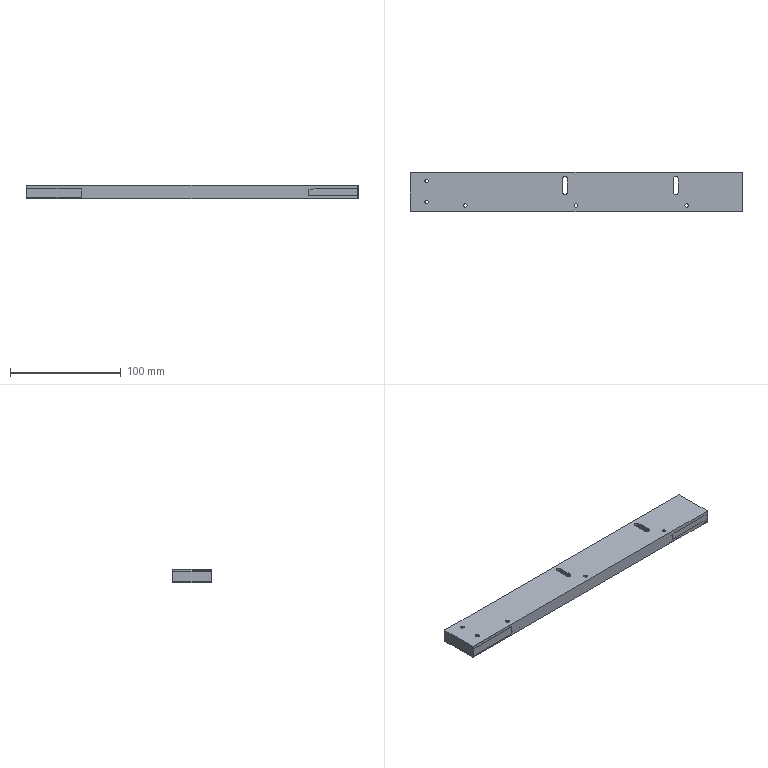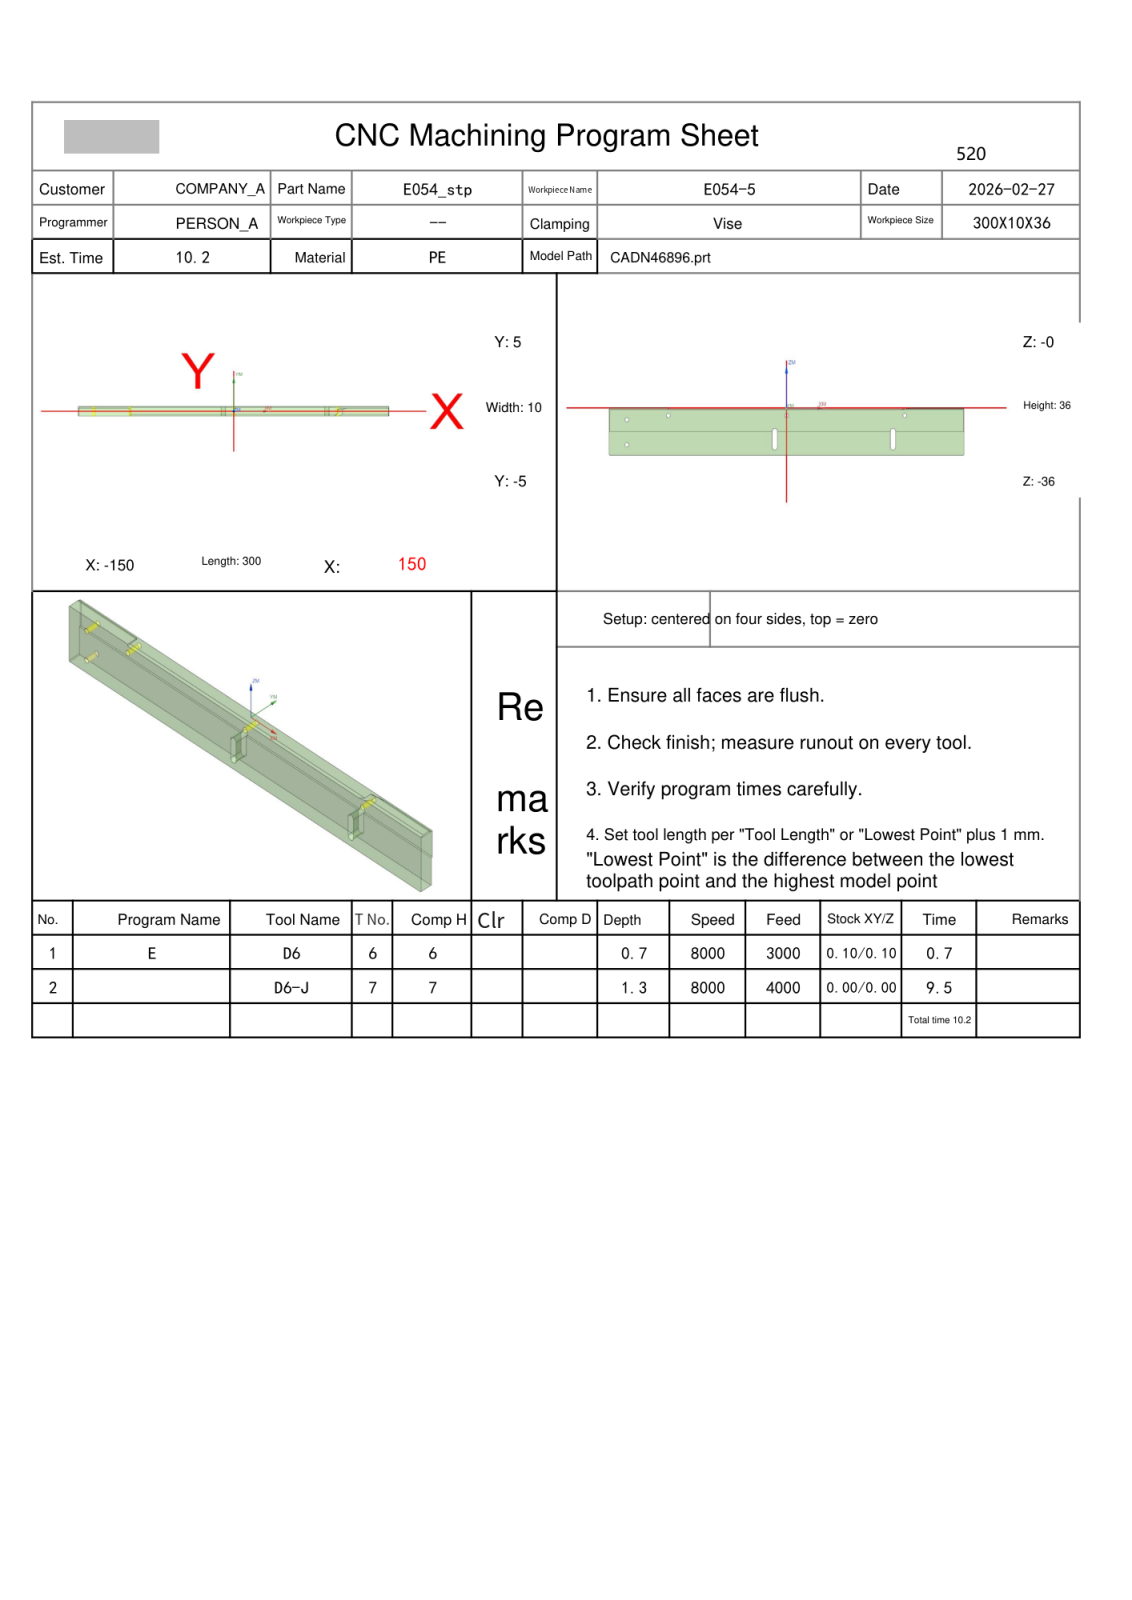NC program | NX | posted by the shop | part box 300 x 36 x 12 mm
Lines 117 to 1396 of 2760:
N2 T07 M06
(D6-J  D=6. R=0. H=07 ce=0.40 di=0.00)
G00 G90 G54 X-1.2 Y8.7 M03 S8000
G43 H07 Z10.4
M08
Z.7
G01 Z-.8 F1000.
Y6.3
G03 X0.0 Y5.1 I1.2 J0.0
G01 X98.232
X98.35 Y4.98
X98.29 Y4.876
X98.157 Y4.803
X97.117 Y3.838
X96.6 Y2.387
Y-3.004
G02 X96.004 Y-3.6 I-.6 J.004
G01 X-96.004
G02 X-96.6 Y-3.004 I.004 J.6
G01 Y4.504
G02 X-96.004 Y5.1 I.6 J-.004
G01 X1.252
G02 X1.675 Y4.925 I-.001 J-.6
G01 X4.325 Y2.275
G03 X4.748 Y2.1 I.424 J.425
G01 X93.004
G02 X93.6 Y1.504 I-.004 J-.6
G01 Y-.004
G02 X93.004 Y-.6 I-.6 J.004
G01 X-93.004
G02 X-93.6 Y-.004 I.004 J.6
G01 Y1.504
G02 X-93.004 Y2.1 I.6 J-.004
G01 X3.
X4.
G03 X5.2 Y3.3 I0.0 J1.2
G01 Y8.7
Z.7
G00 Z10.4
G00 G90 X-154.2 Y7.199 M03 S8000
Z11.2
Z.2
G01 Z-.8 F1000.
G41 D07
Y6.999
G03 X-153. Y5.8 I1.2 J.001
G01 X-97.
Y-6.
G03 X-95.8 Y-7.2 I1.2 J0.0
G01 G40 X-95.6
Z.2
G00 X95.6
G01 Z-.8
G41 D07
X95.8
G03 X97. Y-6. I0.0 J1.2
G01 Y2.09
X97.165 Y2.938
X97.648 Y3.76
X98.146 Y4.267
X98.579 Y4.58
X98.953 Y4.788
X99.287 Y4.938
G02 X100.818 Y5.37 I2.982 J-7.627
G01 X101.137 Y5.429
X101.467 Y5.483
G02 X103.27 Y5.686 I3.532 J-23.309
X106.21 Y5.8 I2.94 J-37.717
G01 X106.326
X153.
G03 X154.2 Y6.999 I0.0 J1.2
G01 G40 Y7.199
Z.2
G00 Z11.2
G00 G90 X96.912 Y-10.137 M03 S8000
Z10.01
Z-.304
G01 Z-.804 F4000.
X97.217 Y-6.067
X97.219 Y-6.025
X97.188 Y-5.992
X97.146 Y-5.99
X-97.151
X-97.176 Y-6.042
Z-.808
X97.127
X97.108 Y-6.058 Z-.812
X-97.182
X-97.188 Y-6.074 Z-.816
X97.089
X97.07 Y-6.09 Z-.82
X-97.194
X-97.201 Y-6.106 Z-.824
X97.051
X97.033 Y-6.122 Z-.828
X-97.207
X-97.213 Y-6.138 Z-.832
X97.015
X96.998 Y-6.154 Z-.836
X-97.22
X-97.227 Y-6.17 Z-.84
X96.98
X96.962 Y-6.186 Z-.844
X-97.234
X-97.24 Y-6.202 Z-.848
X96.945
X96.927 Y-6.218 Z-.852
X-97.247
X-97.255 Y-6.234 Z-.856
X96.91
X96.892 Y-6.25 Z-.86
X-97.262
X-97.269 Y-6.266 Z-.864
X96.875
X96.857 Y-6.282 Z-.868
X-97.277
X-97.284 Y-6.298 Z-.872
X96.84
X96.822 Y-6.314 Z-.876
X-97.292
X-97.3 Y-6.33 Z-.88
X96.805
X96.787 Y-6.346 Z-.884
X-97.308
X-97.316 Y-6.362 Z-.888
X96.769
X96.752 Y-6.378 Z-.892
X-97.324
X-97.332 Y-6.394 Z-.896
X96.734
X96.717 Y-6.41 Z-.9
X-97.341
X-97.349 Y-6.426 Z-.904
X96.7
X96.684 Y-6.442 Z-.908
X-97.358
X-97.367 Y-6.458 Z-.912
X96.668
X96.652 Y-6.474 Z-.916
X-97.376
X-97.385 Y-6.49 Z-.92
X96.637
X96.623 Y-6.506 Z-.924
X-97.394
X-97.403 Y-6.522 Z-.928
X96.608
X96.593 Y-6.538 Z-.932
X-97.413
X-97.422 Y-6.554 Z-.936
X96.579
X96.564 Y-6.57 Z-.94
X-97.432
X-97.442 Y-6.586 Z-.944
X96.549
X96.535 Y-6.602 Z-.948
X-97.452
X-97.462 Y-6.618 Z-.952
X96.52
X96.505 Y-6.634 Z-.956
X-97.472
X-97.483 Y-6.65 Z-.96
X96.49
X96.476 Y-6.666 Z-.964
X-97.493
X-97.504 Y-6.682 Z-.968
X96.461
X96.446 Y-6.698 Z-.972
X-97.515
X-97.526 Y-6.714 Z-.976
X96.432
X96.417 Y-6.73 Z-.98
X-97.537
X-97.548 Y-6.746 Z-.984
X96.402
X96.388 Y-6.762 Z-.988
X-97.56
X-97.571 Y-6.778 Z-.992
X96.373
X96.359 Y-6.794 Z-.996
X-97.583
X-97.595 Y-6.81 Z-1.
X96.347
X96.336 Y-6.826 Z-1.004
X-97.607
X-97.619 Y-6.842 Z-1.008
X96.325
X96.314 Y-6.858 Z-1.012
X-97.632
X-97.645 Y-6.874 Z-1.016
X96.303
X96.292 Y-6.89 Z-1.02
X-97.657
X-97.67 Y-6.906 Z-1.024
X96.281
X96.27 Y-6.922 Z-1.028
X-97.684
X-97.697 Y-6.938 Z-1.032
X96.247
X96.236 Y-6.954 Z-1.036
X-97.71
X-97.724 Y-6.97 Z-1.04
X96.225
X96.214 Y-6.986 Z-1.044
X-97.738
X-97.752 Y-7.002 Z-1.048
X96.203
X96.192 Y-7.018 Z-1.052
X-97.767
X-97.781 Y-7.034 Z-1.056
X96.182
Y-7.05 Z-1.06
X-97.796
X-97.811 Y-7.066 Z-1.064
X96.171
X96.16 Y-7.082 Z-1.068
X-97.826
X-97.842 Y-7.098 Z-1.072
X96.149
X96.138 Y-7.114 Z-1.076
X-97.857
X-97.873 Y-7.13 Z-1.08
X96.127
X96.116 Y-7.146 Z-1.084
X-97.889
X-97.906 Y-7.162 Z-1.088
X96.109
X96.102 Y-7.178 Z-1.092
X-97.922
X-97.939 Y-7.194 Z-1.096
X96.095
X96.088 Y-7.21 Z-1.1
X-97.956
X-97.974 Y-7.226 Z-1.104
X96.082
X96.075 Y-7.242 Z-1.108
X-97.992
X-98.01 Y-7.258 Z-1.112
X96.068
X96.061 Y-7.274 Z-1.116
X-98.028
X-98.047 Y-7.29 Z-1.12
X96.054
X96.048 Y-7.306 Z-1.124
X-98.065
X-98.085 Y-7.322 Z-1.128
X96.041
X96.034 Y-7.338 Z-1.132
X-98.104
X-98.124 Y-7.354 Z-1.136
X96.027
X96.02 Y-7.37 Z-1.14
X-98.144
X-98.165 Y-7.386 Z-1.144
X96.018
X96.015 Y-7.402 Z-1.148
X-98.186
X-98.207 Y-7.418 Z-1.152
X96.012
X96.009 Y-7.434 Z-1.156
X-98.229
X-98.251 Y-7.45 Z-1.16
X96.006
X96.003 Y-7.466 Z-1.164
X-98.274
X-98.297 Y-7.482 Z-1.168
X96.
X95.989 Y-7.498 Z-1.172
X-98.321
X-98.345 Y-7.514 Z-1.176
X95.991
X95.993 Y-7.53 Z-1.18
X-98.369
X-98.394 Y-7.546 Z-1.184
X95.985
X95.987 Y-7.562 Z-1.188
X-98.42
X-98.446 Y-7.578 Z-1.192
X95.989
X95.991 Y-7.594 Z-1.196
X-98.473
X-98.501 Y-7.61 Z-1.2
X95.993
X95.995 Y-7.626 Z-1.204
X-98.529
X-98.558 Y-7.642 Z-1.208
X96.007
X96.009 Y-7.658 Z-1.212
X-98.588
X-98.618 Y-7.674 Z-1.216
X96.02
Y-7.69 Z-1.22
X-98.649
X-98.682 Y-7.706 Z-1.224
X96.029
Y-7.722 Z-1.228
X-98.715
X-98.75 Y-7.738 Z-1.232
X96.041
X96.053 Y-7.754 Z-1.236
X-98.785
X-98.822 Y-7.77 Z-1.24
X96.065
X96.077 Y-7.786 Z-1.244
X-98.861
X-98.901 Y-7.802 Z-1.248
X96.089
X96.113 Y-7.818 Z-1.252
X-98.942
X-98.986 Y-7.834 Z-1.256
X96.139
X96.17 Y-7.85 Z-1.26
X-99.032
X-99.08 Y-7.866 Z-1.264
X96.198
X96.225 Y-7.882 Z-1.268
X-99.132
X-99.187 Y-7.898 Z-1.272
X96.217
X96.251 Y-7.914 Z-1.276
X-99.246
X-99.311 Y-7.93 Z-1.28
X96.317
G00 Z-.784
X99.995 Y-11.01
G01 Z-1.284
Y-8.026
X96.995 Y-8.01
X96.933
X96.861 Y-8.007
X96.769 Y-8.003
X96.367 Y-7.946
X-99.383
X-99.465 Y-7.962 Z-1.288
X96.429
X96.887 Y-8.017
X96.995 Y-8.01
Z-1.3
X96.969 Y-8.067
X96.902
X96.875 Y-8.01
X-100.
G00 Z10.01
G00 G90 X155.82 Y-5.989 M03 S8000
Z10.277
Z.496
G01 Z-.004 F4000.
X150.621
X103.036
X102.955 Y-6.037 Z-.008
X103.051 Y-6.042
X149.508
X150.634 Y-6.041
X150.638 Y-6.057 Z-.012
X149.512 Y-6.058
X103.051
X102.93 Y-6.053
X102.904 Y-6.069 Z-.016
X103.051 Y-6.074
X149.516
X150.643 Y-6.073
X150.647 Y-6.089 Z-.02
X149.52 Y-6.09
X103.051
X102.879 Y-6.086
X102.854 Y-6.103 Z-.024
X103.051 Y-6.106
X149.524
X150.651 Y-6.105
X150.655 Y-6.121 Z-.028
X149.528 Y-6.122
X103.051
X102.829 Y-6.12
X102.804 Y-6.137 Z-.032
X103.051 Y-6.138
X149.532
X150.659 Y-6.137
X150.663 Y-6.153 Z-.036
X149.536 Y-6.154
X103.051
X102.779 Y-6.153
X102.754 Y-6.169 Z-.04
X104.75 Y-6.17
X149.54
X150.667 Y-6.169
X150.671 Y-6.185 Z-.044
X149.544 Y-6.186
X104.725
X102.729
X102.704 Y-6.202 Z-.048
X104.7
X149.548
X150.675
X150.679 Y-6.218 Z-.052
X149.552
X102.705
X102.679 Y-6.216
X102.654 Y-6.231 Z-.056
X102.705 Y-6.234
X149.556
X150.683
X150.687 Y-6.25 Z-.06
X149.56
X102.705
X102.629 Y-6.246
X102.605 Y-6.261 Z-.064
X102.705 Y-6.266
X149.564
X150.691
X150.695 Y-6.282 Z-.068
X149.568
X102.705
X102.58 Y-6.276
X102.555 Y-6.292 Z-.072
X102.705 Y-6.298
X149.572
X150.7
X150.704 Y-6.314 Z-.076
X149.576
X102.705
X102.53 Y-6.308
X102.505 Y-6.324 Z-.08
X102.705 Y-6.33
X149.58
X150.708
X150.712 Y-6.346 Z-.084
X149.584
X102.705
X102.48 Y-6.341
X102.455 Y-6.357 Z-.088
X102.705 Y-6.362
X149.588
X150.716
X150.72 Y-6.378 Z-.092
X149.592
X102.705
X102.43 Y-6.374
X102.405 Y-6.391 Z-.096
X102.705 Y-6.394
X149.596
X150.724
X150.728 Y-6.41 Z-.1
X149.6
X102.705
X102.38 Y-6.409
X102.355 Y-6.426 Z-.104
X104.35
X149.604
X150.732
X150.736 Y-6.441 Z-.108
X149.608 Y-6.442
X102.36
X102.33 Y-6.44
X102.305 Y-6.455 Z-.112
X102.36 Y-6.458
X149.612
X150.74 Y-6.457
X150.744 Y-6.473 Z-.116
X149.616 Y-6.474
X102.36
X102.28 Y-6.472
X102.255 Y-6.487 Z-.12
X102.36 Y-6.49
X150.724
X150.748 Y-6.489
X150.752 Y-6.505 Z-.124
X150.724 Y-6.506
X102.36
X102.23 Y-6.502
X102.205 Y-6.518 Z-.128
X102.36 Y-6.522
X150.724
X150.756 Y-6.52
X150.76 Y-6.536 Z-.132
X150.724 Y-6.538
X102.36
X102.181 Y-6.534
X102.156 Y-6.55 Z-.136
X102.36 Y-6.554
X150.724
X150.764 Y-6.552
X150.768 Y-6.568 Z-.14
X150.724 Y-6.57
X102.36
X102.131 Y-6.567
X102.106 Y-6.583 Z-.144
X102.36 Y-6.586
X150.724
X150.772 Y-6.584
X150.776 Y-6.6 Z-.148
X150.724 Y-6.602
X102.36
X102.081 Y-6.6
X102.056 Y-6.616 Z-.152
X102.36 Y-6.618
X150.724
X150.78 Y-6.616
X150.784 Y-6.632 Z-.156
X150.724 Y-6.634
X104.025
X102.031 Y-6.633
X102.006 Y-6.649 Z-.16
X104. Y-6.65
X150.724
X150.788 Y-6.648
X150.793 Y-6.663 Z-.164
X150.724 Y-6.666
X102.014
X101.982 Y-6.664
X101.957 Y-6.678 Z-.168
X102.014 Y-6.682
X150.724
X150.797 Y-6.679
X150.801 Y-6.695 Z-.172
X150.724 Y-6.698
X102.014
X101.932 Y-6.693
X101.907 Y-6.709 Z-.176
X102.014 Y-6.714
X150.724
X150.805 Y-6.711
X150.809 Y-6.727 Z-.18
X150.724 Y-6.73
X102.014
X101.883 Y-6.724
X101.858 Y-6.741 Z-.184
X102.014 Y-6.746
X150.724
X150.813 Y-6.743
X150.817 Y-6.759 Z-.188
X150.724 Y-6.762
X102.014
X101.833 Y-6.757
X101.808 Y-6.774 Z-.192
X102.014 Y-6.778
X150.724
X150.821 Y-6.775
X150.825 Y-6.791 Z-.196
X150.724 Y-6.794
X102.014
X101.783 Y-6.791
X101.758 Y-6.809 Z-.2
X103.75 Y-6.81
X150.724
X150.829 Y-6.808
X150.833 Y-6.823 Z-.204
X150.724 Y-6.826
X103.725
X101.733 Y-6.825
X101.709 Y-6.841 Z-.208
X103.7 Y-6.842
X150.724
X150.837 Y-6.839
X150.841 Y-6.855 Z-.212
X150.724 Y-6.858
X103.675
X101.684
X101.659 Y-6.873 Z-.216
X103.65 Y-6.874
X150.724
X150.845 Y-6.871
X150.849 Y-6.887 Z-.22
X150.724 Y-6.89
X101.669
X101.635 Y-6.888
X101.61 Y-6.903 Z-.224
X101.669 Y-6.906
X150.724
X150.853 Y-6.903
X150.857 Y-6.919 Z-.228
X150.724 Y-6.922
X101.669
X101.585 Y-6.918
X101.56 Y-6.933 Z-.232
X101.669 Y-6.938
X150.724
X150.861 Y-6.935
X150.865 Y-6.951 Z-.236
X150.724 Y-6.954
X101.669
X101.536 Y-6.949
X101.511 Y-6.964 Z-.24
X101.669 Y-6.97
X150.724
X150.869 Y-6.967
X150.873 Y-6.983 Z-.244
X150.724 Y-6.986
X101.669
X101.486 Y-6.98
X101.461 Y-6.997 Z-.248
X101.669 Y-7.002
X150.724
X150.877 Y-6.999
X150.881 Y-7.015 Z-.252
X150.724 Y-7.018
X101.669
X101.437 Y-7.013
X101.412 Y-7.03 Z-.256
X101.669 Y-7.034
X150.724
X150.885 Y-7.031
X150.889 Y-7.047 Z-.26
X150.724 Y-7.05
X101.669
X101.387 Y-7.047
X101.362 Y-7.064 Z-.264
X101.669 Y-7.066
X150.724
X150.893 Y-7.063
X150.897 Y-7.079 Z-.268
X150.724 Y-7.082
X103.325
X101.338 Y-7.081
X101.313 Y-7.097 Z-.272
X103.3 Y-7.098
X150.724
X150.901 Y-7.095
X150.905 Y-7.112 Z-.276
X150.724 Y-7.114
X101.323
X101.288 Y-7.112
X101.263 Y-7.127 Z-.28
X101.323 Y-7.13
X150.724
X150.909 Y-7.128
X150.913 Y-7.144 Z-.284
X150.724 Y-7.146
X101.323
X101.239 Y-7.143
X101.214 Y-7.159 Z-.288
X101.323 Y-7.162
X150.724
X150.917 Y-7.16
X150.921 Y-7.176 Z-.292
X150.724 Y-7.178
X101.323
X101.189 Y-7.175
X101.164 Y-7.191 Z-.296
X101.323 Y-7.194
X150.724
X150.924 Y-7.192
X150.928 Y-7.208 Z-.3
X150.724 Y-7.21
X101.323
X101.14 Y-7.207
X101.115 Y-7.223 Z-.304
X101.323 Y-7.226
X150.724
X150.932 Y-7.224
X150.936 Y-7.24 Z-.308
X150.724 Y-7.242
X101.323
X101.09 Y-7.239
X101.065 Y-7.255 Z-.312
X101.323 Y-7.258
X150.724
X150.94 Y-7.256
X150.944 Y-7.272 Z-.316
X150.724 Y-7.274
X101.323
X101.041 Y-7.272
X101.016 Y-7.289 Z-.32
X101.323 Y-7.29
X150.724
X150.948 Y-7.288
X150.952 Y-7.304 Z-.324
X149.824 Y-7.306
X102.975
X100.991 Y-7.305
X100.966 Y-7.321 Z-.328
X102.95 Y-7.322
X149.828
X150.956 Y-7.32
X150.96 Y-7.336 Z-.332
X149.832 Y-7.338
X100.978
X100.942 Y-7.335
X100.917 Y-7.35 Z-.336
X100.978 Y-7.354
X149.836
X150.964 Y-7.353
X150.968 Y-7.369 Z-.34
X149.84 Y-7.37
X100.978
X100.892 Y-7.365
X100.868 Y-7.38 Z-.344
X100.978 Y-7.386
X149.844
X150.972 Y-7.385
X150.976 Y-7.401 Z-.348
X149.848 Y-7.402
X100.978
X100.843 Y-7.396
X100.818 Y-7.412 Z-.352
X100.978 Y-7.418
X149.852
X150.98 Y-7.417
X150.984 Y-7.433 Z-.356
X149.856 Y-7.434
X100.978
X100.793 Y-7.429
X100.768 Y-7.446 Z-.36
X100.978 Y-7.45
X149.86
X150.988 Y-7.449
X150.992 Y-7.465 Z-.364
X149.864 Y-7.466
X100.978
X100.744 Y-7.463
X100.719 Y-7.48 Z-.368
X100.978 Y-7.482
X149.868
X150.996 Y-7.481
X151. Y-7.497 Z-.372
X149.872 Y-7.498
X102.675
X100.694 Y-7.497
X100.669 Y-7.514 Z-.376
X102.65
X149.876
X151.004 Y-7.513
X151.008 Y-7.529 Z-.38
X149.88 Y-7.53
X102.625
X100.645
X100.63 Y-7.546 Z-.384
X102.6
X149.884
X151.011 Y-7.545
X151.015 Y-7.561 Z-.388
X149.888 Y-7.562
X102.575
X100.626
X100.622 Y-7.577 Z-.392
X102.55 Y-7.578
X149.892
X151.019 Y-7.577
X151.023 Y-7.594 Z-.396
X149.896
X102.525
X100.617 Y-7.593
X100.613 Y-7.609 Z-.4
X100.632 Y-7.61
X149.9
X151.027
X151.031 Y-7.626 Z-.404
X149.904
X100.632
X100.609 Y-7.625
X100.604 Y-7.64 Z-.408
X100.632 Y-7.642
X149.908
X151.035
X151.039 Y-7.658 Z-.412
X149.912
X100.632
X100.6 Y-7.656
X100.596 Y-7.672 Z-.416
X100.632 Y-7.674
X149.916
X151.043
X151.047 Y-7.69 Z-.42
X149.92
X100.632
X100.591 Y-7.688
X100.587 Y-7.704 Z-.424
X100.632 Y-7.706
X149.924
X151.051
X151.055 Y-7.722 Z-.428
X149.928
X100.632
X100.583 Y-7.72
X100.578 Y-7.735 Z-.432
X100.632 Y-7.738
X149.932
X151.059
X151.063 Y-7.754 Z-.436
X149.936
X100.632
X100.574 Y-7.751
X100.57 Y-7.767 Z-.44
X100.632 Y-7.77
X149.94
X151.067
X151.071 Y-7.786 Z-.444
X149.944
X100.632
X100.565 Y-7.783
X100.561 Y-7.799 Z-.448
X100.632 Y-7.802
X149.948
X151.075
X151.079 Y-7.818 Z-.452
X149.952
X100.632
X100.556 Y-7.815
X100.554 Y-7.833 Z-.456
X102.15 Y-7.834
X149.956
X151.083
X151.086 Y-7.849 Z-.46
X149.96 Y-7.85
X100.632
X100.562 Y-7.847
X100.571 Y-7.864 Z-.464
X100.632 Y-7.866
X151.07
X151.09 Y-7.865
X151.094 Y-7.881 Z-.468
X151.07 Y-7.882
X100.632
X100.579 Y-7.88
X100.588 Y-7.896 Z-.472
X100.632 Y-7.898
X151.07
X151.098 Y-7.897
X151.102 Y-7.912 Z-.476
X151.07 Y-7.914
X100.632
X100.596 Y-7.912
X100.605 Y-7.929 Z-.48
X100.632 Y-7.93
X151.07
X151.106 Y-7.928
X151.11 Y-7.944 Z-.484
X151.07 Y-7.946
X100.632
X100.613 Y-7.945
X100.622 Y-7.961 Z-.488
X102.014 Y-7.962
X151.07
X151.114 Y-7.96
X151.126 Y-8.008 Z-.5
X100.647 Y-8.01
G00 Z10.277
G00 G90 X102.027 Y-9.47 M03 S8000
Z10.846
Z.496
G01 Z-.004 F4000.
X102.024 Y-4.268
X102.021 Y1.757
Y1.774
G02 X103.421 Y4.458 I3.273 J0.0
X104.87 Y5.141 I2.871 J-4.214
X107.038 Y5.568 I3.835 J-13.761
X111.235 Y5.811 I4.197 J-36.119
G01 X111.466 Y5.81
Z-.008
X111.2 Y5.811
G03 X107.038 Y5.577 I0.0 J-37.093
X104.619 Y5.082 I1.368 J-12.85
X102.933 Y4.117 I1.18 J-4.017
X101.94 Y1.8 I2.236 J-2.33
G01 Y-3.032
X101.942 Y-4.321
X101.917 Y-4.338 Z-.012
X101.915 Y-3.048
Y1.8
G02 X103.315 Y4.458 I3.28 J-.03
X104.764 Y5.141 I2.789 J-4.039
X107.384 Y5.618 I4.025 J-14.675
X111.203 Y5.811 I3.819 J-37.674
G01 X111.466 Y5.81
Z-.016
X111.198 Y5.811
G03 X107.384 Y5.621 I0.0 J-38.304
X104.739 Y5.141 I1.4 J-15.25
X103.29 Y4.458 I1.377 J-4.801
X101.89 Y1.8 I1.88 J-2.688
G01 Y-3.064
X101.891 Y-4.354
X101.866 Y-4.37 Z-.02
X101.865 Y-3.08
Y1.8
G02 X103.265 Y4.458 I3.28 J-.03
X104.715 Y5.141 I2.845 J-4.159
X107.038 Y5.585 I3.891 J-14.055
X111.138 Y5.811 I4.1 J-37.013
X111.466 Y5.81 I0.0 J-37.239
G01 Z-.024
G03 X111.17 Y5.811 I-.296 J-38.84
X107.384 Y5.626 I0.0 J-38.841
G01 X107.038 Y5.588
G03 X104.69 Y5.141 I1.542 J-14.502
X103.24 Y4.458 I1.413 J-4.879
X101.84 Y1.8 I1.88 J-2.688
G01 Y-3.096
Y-4.387
X101.815 Y-4.403 Z-.028
Y-3.112
Y1.801
G02 X103.319 Y4.525 I3.218 J0.0
X104.779 Y5.171 I2.723 J-4.183
G01 X105.31 Y5.31
G02 X107.384 Y5.629 I3.827 J-17.979
X111.156 Y5.811 I3.772 J-38.935
X111.466 Y5.81 I0.0 J-39.117
G01 Z-.032
G03 X111.105 Y5.812 I-.361 J-37.981
X107.038 Y5.593 I0.0 J-37.983
X104.64 Y5.141 I1.458 J-14.313
X103.19 Y4.458 I1.433 J-4.921
X101.79 Y1.8 I1.879 J-2.688
G01 Y-3.128
Y-4.42
X101.765 Y-4.435 Z-.036
Y-3.144
Y1.8
G02 X103.165 Y4.458 I3.279 J-.03
X104.615 Y5.141 I2.901 J-4.278
X107.038 Y5.596 I3.908 J-14.129
X111.089 Y5.812 I4.051 J-37.935
X111.466 Y5.81 I0.0 J-38.15
G01 Z-.04
G03 X111.074 Y5.812 I-.392 J-38.323
X107.038 Y5.599 I0.0 J-38.325
X104.758 Y5.186 I1.511 J-14.853
X103.221 Y4.511 I1.363 J-5.191
X101.74 Y1.8 I1.741 J-2.711
G01 Y-3.16
Y-4.452
X101.715 Y-4.468 Z-.044
Y-3.176
Y1.8
G02 X103.205 Y4.517 I3.222 J0.0
X104.752 Y5.191 I2.909 J-4.564
X107.038 Y5.602 I3.823 J-14.709
X111.058 Y5.812 I4.02 J-38.291
X111.466 Y5.81 I0.0 J-38.501
G01 Z-.048
G03 X111.093 Y5.812 I-.374 J-40.792
X107.384 Y5.643 I0.0 J-40.794
X104.852 Y5.225 I1.525 J-17.116
X103.202 Y4.53 I1.326 J-5.459
X101.69 Y1.803 I1.704 J-2.727
G01 Y-3.192
Y-4.484
X101.665 Y-4.5 Z-.052
Y-3.208
Y1.801
G02 X103.185 Y4.535 I3.218 J0.0
X104.861 Y5.234 I2.991 J-4.814
X107.384 Y5.646 I4.102 J-17.2
X111.061 Y5.812 I3.677 J-40.526
X111.466 Y5.81 I0.0 J-40.692
G01 Z-.056
G03 X111.057 Y5.812 I-.409 J-41.112
X107.384 Y5.648 I0.0 J-41.114
X104.965 Y5.265 I1.604 J-17.967
G01 X104.491 Y5.141
G03 X103.13 Y4.516 I1.531 J-5.126
X101.64 Y1.803 I1.725 J-2.713
G01 Y-3.224
Y-4.517
X101.615 Y-4.533 Z-.06
Y-3.24
Y1.801
G02 X103.117 Y4.523 I3.219 J0.0
X104.965 Y5.271 I3.002 J-4.76
X107.384 Y5.65 I4.043 J-17.929
X111.05 Y5.812 I3.666 J-41.283
X111.466 Y5.81 I0.0 J-41.446
G01 Z-.064
G03 X111.03 Y5.812 I-.436 J-41.437
X107.384 Y5.652 I0.0 J-41.439
X104.965 Y5.278 I1.645 J-18.662
X103.095 Y4.525 I1.153 J-5.562
X101.59 Y1.802 I1.712 J-2.723
G01 Y-3.256
X101.591 Y-4.549
X101.566 Y-4.565 Z-.068
X101.565 Y-3.272
Y1.802
G02 X103.05 Y4.513 I3.216 J0.0
X104.416 Y5.141 I2.95 J-4.614
G01 X104.965 Y5.284
G02 X107.384 Y5.654 I4.087 J-18.662
X111.016 Y5.812 I3.632 J-41.435
X111.466 Y5.81 I0.0 J-41.594
G01 Z-.072
G03 X110.995 Y5.813 I-.471 J-41.577
X107.384 Y5.656 I0.0 J-41.579
X104.965 Y5.291 I1.691 J-19.416
G01 X104.391 Y5.141
G03 X103.027 Y4.514 I1.547 J-5.163
X101.54 Y1.803 I1.727 J-2.71
G01 Y-3.288
Y-4.581
X101.515 Y-4.597 Z-.076
Y-3.304
Y1.801
G02 X103.016 Y4.522 I3.217 J0.0
X104.965 Y5.297 I3.054 J-4.842
X107.384 Y5.658 I4.134 J-19.458
X110.981 Y5.813 I3.597 J-41.577
X111.466 Y5.81 I0.0 J-41.732
G01 Z-.08
G03 X111.021 Y5.812 I-.445 J-44.838
X108.075 Y5.715 I0.0 J-44.84
X104.965 Y5.304 I1.33 J-22.011
X103. Y4.528 I1.111 J-5.69
X101.49 Y1.801 I1.707 J-2.727
G01 Y-4.419
X101.492 Y-4.613
X101.467 Y-4.629 Z-.084
X101.465 Y-4.419
Y1.8
G02 X102.984 Y4.533 I3.218 J0.0
X104.965 Y5.31 I3.097 J-4.98
X107.384 Y5.661 I4.186 J-20.325
X110.919 Y5.814 I3.535 J-40.983
X111.466 Y5.81 I0.0 J-41.135
G01 Z-.088
X110.149 Y5.802
G03 X105.851 Y5.482 I.231 J-32.202
X103.928 Y5.015 I1.438 J-10.11
X102.433 Y4.117 I1.318 J-3.885
X101.44 Y1.8 I2.238 J-2.33
G01 Y-4.419
X101.442 Y-4.646
X101.417 Y-4.662 Z-.092
X101.415 Y-4.419
Y1.8
G02 X102.408 Y4.117 I3.231 J-.014
X103.928 Y5.024 I2.816 J-2.991
X105.826 Y5.482 I3.375 J-9.813
X109.457 Y5.79 I4.509 J-31.679
X111.097 Y5.811 I1.64 J-62.495
X111.466 Y5.81 I0.0 J-62.516
G01 Z-.096
G03 X111.048 Y5.812 I-.418 J-55.815
X109.112 Y5.778 I0.0 J-55.816
X105.801 Y5.482 I1.126 J-31.302
X103.928 Y5.033 I1.518 J-10.445
X102.383 Y4.117 I1.272 J-3.908
X101.39 Y1.8 I2.238 J-2.33
G01 Y-3.384
X101.392 Y-4.678
X101.366 Y-4.694 Z-.1
X101.365 Y-3.4
Y1.8
G02 X102.358 Y4.117 I3.231 J-.014
X103.928 Y5.041 I2.823 J-2.999
X105.776 Y5.482 I3.41 J-10.189
X109.112 Y5.779 I4.443 J-31.072
X111.044 Y5.812 I1.932 J-57.197
X111.466 Y5.81 I0.0 J-57.23
G01 Z-.104
G03 X111.008 Y5.812 I-.458 J-54.908
X108.7 Y5.763 I0.0 J-54.91
X106.574 Y5.586 I1.084 J-25.76
G01 X105.986 Y5.512
G03 X103.848 Y5.024 I1.372 J-10.934
X102.333 Y4.117 I1.316 J-3.918
X101.34 Y1.8 I2.238 J-2.33
G01 Y-3.416
X101.341 Y-4.71
X101.316 Y-4.726 Z-.108
X101.315 Y-3.432
Y1.8
G02 X102.308 Y4.117 I3.231 J-.014
X103.928 Y5.058 I2.841 J-3.023
X105.727 Y5.482 I3.452 J-10.615
X109.457 Y5.791 I4.469 J-31.286
X111.104 Y5.811 I1.646 J-69.13
G01 X111.466 Y5.81
Z-.112
G03 X110.849 Y5.814 I-.617 J-43.252
X107.384 Y5.675 I0.0 J-43.257
X104.619 Y5.265 I1.502 J-19.645
X102.776 Y4.513 I1.147 J-5.445
X101.29 Y1.804 I1.727 J-2.709
G01 Y-3.448
Y-4.742
X101.265 Y-4.759 Z-.116
Y-3.464
Y1.8
G02 X102.891 Y4.593 I3.238 J-.016
X103.845 Y5.049 I2.185 J-3.344
X105.677 Y5.482 I3.585 J-11.065
X109.457 Y5.792 I4.499 J-31.677
X111.078 Y5.811 I1.621 J-69.703
X111.466 Y5.81 I0.0 J-69.722
G01 Z-.12
G03 X110.823 Y5.815 I-.643 J-43.732
X107.384 Y5.679 I0.0 J-43.737
X104.619 Y5.278 I1.504 J-20.088
X102.74 Y4.521 I1.145 J-5.556
X101.24 Y1.802 I1.714 J-2.719
G01 Y-3.48
X101.241 Y-4.775
X101.217 Y-4.791 Z-.124
X101.215 Y-4.761
Y1.801
G02 X102.692 Y4.507 I3.218 J0.0
X104.619 Y5.285 I3.006 J-4.672
X107.73 Y5.709 I4.444 J-20.949
X110.854 Y5.814 I3.125 J-46.506
X111.466 Y5.81 I0.0 J-46.61
G01 Z-.128
G03 X110.844 Y5.814 I-.623 J-47.134
X107.73 Y5.711 I0.0 J-47.138
X104.619 Y5.291 I1.346 J-21.686
X102.672 Y4.51 I1.083 J-5.519
X101.19 Y1.803 I1.732 J-2.707
G01 Y-4.761
X101.192 Y-4.807
X101.167 Y-4.823 Z-.132
X101.165 Y-4.761
Y1.802
G02 X102.66 Y4.518 I3.215 J0.0
X104.619 Y5.297 I3.052 J-4.821
X107.73 Y5.713 I4.469 J-21.593
X110.829 Y5.814 I3.099 J-47.436
X111.466 Y5.81 I0.0 J-47.538
G01 Z-.136
G03 X110.821 Y5.814 I-.646 J-48.193
X107.73 Y5.715 I0.0 J-48.197
X104.619 Y5.304 I1.376 J-22.38
X102.64 Y4.521 I1.1 J-5.672
X101.14 Y1.803 I1.711 J-2.717
G01 Y-4.761
X101.143 Y-4.839
X101.118 Y-4.855 Z-.14
X101.115 Y-4.761
Y1.801
G02 X102.628 Y4.529 I3.216 J0.0
X104.619 Y5.31 I3.095 J-4.957
X107.73 Y5.717 I4.524 J-22.501
X110.793 Y5.815 I3.063 J-48.009
X111.466 Y5.81 I0.0 J-48.107
G01 Z-.144
G03 X110.949 Y5.812 I-.517 J-74.642
X109.112 Y5.789 I0.0 J-74.644
X105.503 Y5.482 I.966 J-32.736
X103.583 Y5.017 I1.459 J-10.206
X102.083 Y4.117 I1.307 J-3.878
X101.09 Y1.8 I2.24 J-2.331
G01 Y-4.761
X101.093 Y-4.871
X101.068 Y-4.887 Z-.148
X101.065 Y-4.761
Y1.8
G02 X102.058 Y4.117 I3.233 J-.014
X103.583 Y5.025 I2.811 J-2.985
X105.478 Y5.482 I3.396 J-9.919
X109.112 Y5.79 I4.561 J-32.304
X110.935 Y5.812 I1.823 J-74.542
X111.466 Y5.81 I0.0 J-74.564
G01 Z-.152
G03 X110.92 Y5.812 I-.546 J-74.483
X109.112 Y5.79 I0.0 J-74.485
X105.453 Y5.482 I.887 J-32.45
X103.583 Y5.034 I1.542 J-10.552
X102.033 Y4.117 I1.267 J-3.91
X101.04 Y1.8 I2.24 J-2.331
G01 Y-4.761
X101.043 Y-4.903
X101.018 Y-4.919 Z-.156
X101.015 Y-4.761
Y1.8
G02 X102.008 Y4.117 I3.233 J-.014
X103.583 Y5.042 I2.824 J-3.003
X105.429 Y5.482 I3.432 J-10.3
X109.112 Y5.79 I4.514 J-31.792
X110.906 Y5.812 I1.794 J-74.384
X111.466 Y5.81 I0.0 J-74.405
G01 Z-.16
G03 X110.906 Y5.812 I-.56 J-76.191
X109.112 Y5.791 I0.0 J-76.193
X105.404 Y5.482 I.795 J-31.984
X103.583 Y5.051 I1.632 J-10.941
X101.983 Y4.117 I1.233 J-3.948
X100.99 Y1.8 I2.24 J-2.331
G01 Y-4.761
X100.993 Y-4.934
X100.968 Y-4.95 Z-.164
X100.965 Y-4.761
Y1.8
G02 X102.546 Y4.565 I3.235 J-.015
X103.485 Y5.028 I2.171 J-3.22
X105.602 Y5.51 I3.495 J-10.45
G01 X106.002 Y5.561
G02 X108.421 Y5.768 I3.422 J-25.764
X110.871 Y5.813 I2.45 J-66.875
X111.466 Y5.81 I0.0 J-66.92
G01 Z-.168
G03 X110.927 Y5.812 I-.539 J-82.618
X109.112 Y5.792 I0.0 J-82.619
X106.002 Y5.564 I.579 J-29.253
G01 X105.575 Y5.51
G03 X103.467 Y5.031 I1.382 J-10.963
X102.546 Y4.58 I1.211 J-3.64
X100.94 Y1.8 I1.629 J-2.795
G01 Y-4.761
X100.943 Y-4.966
X100.918 Y-4.982 Z-.172
X100.915 Y-4.761
Y1.8
G02 X102.546 Y4.595 I3.237 J-.016
X103.513 Y5.054 I2.206 J-3.397
X105.519 Y5.51 I3.604 J-11.22
X109.07 Y5.791 I4.246 J-31.026
X110.917 Y5.812 I1.847 J-83.327
X111.466 Y5.81 I0.0 J-83.348
G01 Z-.176
G03 X110.907 Y5.812 I-.559 J-84.087
X109.112 Y5.793 I0.0 J-84.089
X105.522 Y5.513 I.688 J-31.956
X103.654 Y5.115 I1.698 J-12.574
X102.663 Y4.681 I1.187 J-4.053
G01 X102.293 Y4.458
G03 X100.89 Y1.8 I1.863 J-2.683
G01 Y-4.761
X100.892 Y-4.998
X100.867 Y-5.014 Z-.18
X100.865 Y-3.72
Y1.8
G02 X102.268 Y4.458 I3.266 J-.025
G01 X102.635 Y4.679
G02 X103.634 Y5.117 I2.193 J-3.643
X105.498 Y5.513 I3.562 J-12.177
X109.112 Y5.793 I4.277 J-31.683
X110.898 Y5.812 I1.786 J-84.95
X111.466 Y5.81 I0.0 J-84.969
G01 Z-.184
G03 X110.885 Y5.812 I-.581 J-85.456
X109.112 Y5.794 I0.0 J-85.458
X105.255 Y5.482 I.627 J-31.832
X103.696 Y5.141 I2.416 J-14.766
X102.546 Y4.64 I1.179 J-4.275
G01 X102.244 Y4.458
G03 X100.84 Y1.8 I1.862 J-2.683
G01 Y-3.736
X100.841 Y-5.03
X100.815 Y-5.046 Z-.188
Y-3.752
Y1.8
G02 X102.219 Y4.458 I3.265 J-.024
G01 X102.546 Y4.655
G02 X103.671 Y5.141 I2.342 J-3.876
X105.23 Y5.482 I3.964 J-14.373
X109.112 Y5.794 I4.482 J-31.502
X110.873 Y5.812 I1.761 J-85.934
X111.466 Y5.81 I0.0 J-85.952
G01 Z-.192
G03 X110.866 Y5.812 I-.6 J-87.402
X109.112 Y5.794 I0.0 J-87.404
X105.205 Y5.482 I.573 J-31.784
X103.646 Y5.141 I2.382 J-14.607
X102.546 Y4.67 I1.261 J-4.465
G01 X102.194 Y4.458
G03 X100.79 Y1.8 I1.861 J-2.682
G01 Y-3.768
Y-5.062
X100.765 Y-5.078 Z-.196
Y-3.784
Y1.8
G02 X102.169 Y4.458 I3.264 J-.024
X103.621 Y5.141 I2.93 J-4.346
X105.18 Y5.482 I3.907 J-14.109
X108.766 Y5.788 I4.538 J-32.013
X110.785 Y5.813 I2.019 J-83.732
X111.466 Y5.81 I0.0 J-83.756
G01 Z-.2
G03 X110.782 Y5.813 I-.685 J-86.356
X108.766 Y5.789 I0.0 J-86.359
X105.155 Y5.482 I.925 J-32.29
X103.237 Y5.018 I1.472 J-10.268
X101.733 Y4.117 I1.306 J-3.887
X100.74 Y1.8 I2.241 J-2.332
G01 Y-3.8
Y-5.094
X100.715 Y-5.11 Z-.204
Y-3.816
Y1.8
G02 X101.708 Y4.117 I3.234 J-.015
X103.237 Y5.026 I2.814 J-2.992
X105.131 Y5.482 I3.404 J-9.971
X108.766 Y5.79 I4.52 J-31.824